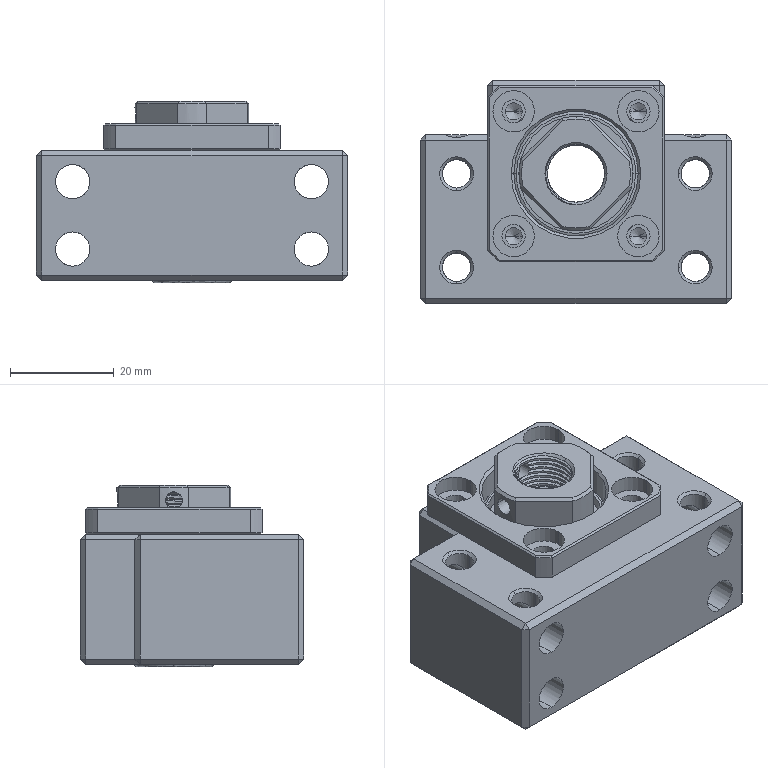Part | STEP file | Screw support seat BK12 | 35 solids | 485 faces | box 60 x 43 x 35 mm | volume 48236 mm3 | spline 153 | cylinder 152 | plane 103 | cone 77 | commonest cylinder face diameters 11 x25 5.5 x24 3.3 x12 22 x9 4.5 x8 6.6 x8